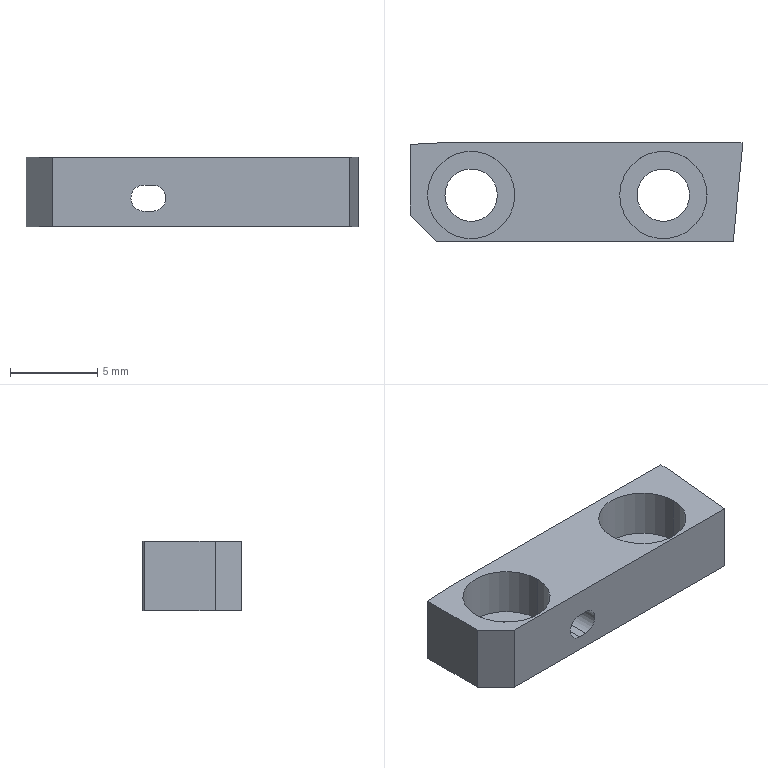Part | NX | 1 solid | 24 faces | box 19 x 5.65 x 4 mm | volume 278.189 mm3 | plane 13 | cylinder 11 | commonest cylinder face diameters 3 x4 5 x4 1.5 x3
STEP:
#1=CARTESIAN_POINT('',(18.5,0.,4.));
#2=VERTEX_POINT('',#1);
#3=CARTESIAN_POINT('',(18.5,0.,0.));
#4=VERTEX_POINT('',#3);
#5=CARTESIAN_POINT('',(18.5,0.,0.));
#6=DIRECTION('',(0.,0.,-1.));
#7=VECTOR('',#6,1000.);
#8=LINE('',#5,#7);
#9=EDGE_CURVE('',#2,#4,#8,.T.);
#10=ORIENTED_EDGE('',*,*,#9,.F.);
#11=CARTESIAN_POINT('',(1.5,0.,4.));
#12=VERTEX_POINT('',#11);
#13=CARTESIAN_POINT('',(0.,0.,4.));
#14=DIRECTION('',(-1.,0.,0.));
#15=VECTOR('',#14,1000.);
#16=LINE('',#13,#15);
#17=EDGE_CURVE('',#2,#12,#16,.T.);
#18=ORIENTED_EDGE('',*,*,#17,.T.);
#19=CARTESIAN_POINT('',(1.5,0.,0.));
#20=VERTEX_POINT('',#19);
#21=CARTESIAN_POINT('',(1.5,0.,0.));
#22=DIRECTION('',(0.,0.,1.));
#23=VECTOR('',#22,1000.);
#24=LINE('',#21,#23);
#25=EDGE_CURVE('',#20,#12,#24,.T.);
#26=ORIENTED_EDGE('',*,*,#25,.F.);
#27=CARTESIAN_POINT('',(0.,0.,0.));
#28=DIRECTION('',(1.,0.,0.));
#29=VECTOR('',#28,1000.);
#30=LINE('',#27,#29);
#31=EDGE_CURVE('',#20,#4,#30,.T.);
#32=ORIENTED_EDGE('',*,*,#31,.T.);
#33=EDGE_LOOP('',(#10,#18,#26,#32));
#34=FACE_BOUND('',#33,.T.);
#35=CARTESIAN_POINT('',(7.25,0.,2.4));
#36=VERTEX_POINT('',#35);
#37=CARTESIAN_POINT('',(7.25,0.,0.9));
#38=VERTEX_POINT('',#37);
#39=CARTESIAN_POINT('',(7.25,0.,1.65));
#40=DIRECTION('',(0.,1.,0.));
#41=DIRECTION('',(-1.,0.,0.));
#42=AXIS2_PLACEMENT_3D('',#39,#40,#41);
#43=CIRCLE('',#42,0.75);
#44=EDGE_CURVE('',#36,#38,#43,.T.);
#45=ORIENTED_EDGE('',*,*,#44,.T.);
#46=CARTESIAN_POINT('',(6.75,0.,0.9));
#47=VERTEX_POINT('',#46);
#48=CARTESIAN_POINT('',(0.,0.,0.9));
#49=DIRECTION('',(-1.,0.,0.));
#50=VECTOR('',#49,1000.);
#51=LINE('',#48,#50);
#52=EDGE_CURVE('',#38,#47,#51,.T.);
#53=ORIENTED_EDGE('',*,*,#52,.T.);
#54=CARTESIAN_POINT('',(6.,0.,1.65));
#55=VERTEX_POINT('',#54);
#56=CARTESIAN_POINT('',(6.75,0.,1.65));
#57=DIRECTION('',(0.,1.,0.));
#58=DIRECTION('',(-1.,0.,0.));
#59=AXIS2_PLACEMENT_3D('',#56,#57,#58);
#60=CIRCLE('',#59,0.75);
#61=EDGE_CURVE('',#47,#55,#60,.T.);
#62=ORIENTED_EDGE('',*,*,#61,.T.);
#63=CARTESIAN_POINT('',(6.75,0.,2.4));
#64=VERTEX_POINT('',#63);
#65=CARTESIAN_POINT('',(6.75,0.,1.65));
#66=DIRECTION('',(0.,1.,0.));
#67=DIRECTION('',(-1.,0.,0.));
#68=AXIS2_PLACEMENT_3D('',#65,#66,#67);
#69=CIRCLE('',#68,0.75);
#70=EDGE_CURVE('',#55,#64,#69,.T.);
#71=ORIENTED_EDGE('',*,*,#70,.T.);
#72=CARTESIAN_POINT('',(0.,0.,2.4));
#73=DIRECTION('',(1.,0.,0.));
#74=VECTOR('',#73,1000.);
#75=LINE('',#72,#74);
#76=EDGE_CURVE('',#64,#36,#75,.T.);
#77=ORIENTED_EDGE('',*,*,#76,.T.);
#78=EDGE_LOOP('',(#45,#53,#62,#71,#77));
#79=FACE_BOUND('',#78,.T.);
#80=CARTESIAN_POINT('',(0.,0.,0.));
#81=DIRECTION('',(0.,-1.,0.));
#82=DIRECTION('',(0.,0.,-1.));
#83=AXIS2_PLACEMENT_3D('',#80,#81,#82);
#84=PLANE('',#83);
#85=ADVANCED_FACE('',(#34,#79),#84,.T.);
#86=CARTESIAN_POINT('',(19.,5.15,0.));
#87=VERTEX_POINT('',#86);
#88=CARTESIAN_POINT('',(18.5,0.,0.));
#89=DIRECTION('',(-0.09663,-0.9953,0.));
#90=VECTOR('',#89,1000.);
#91=LINE('',#88,#90);
#92=EDGE_CURVE('',#87,#4,#91,.T.);
#93=ORIENTED_EDGE('',*,*,#92,.T.);
#94=ORIENTED_EDGE('',*,*,#31,.F.);
#95=CARTESIAN_POINT('',(0.,1.5,0.));
#96=VERTEX_POINT('',#95);
#97=CARTESIAN_POINT('',(1.5,0.,0.));
#98=DIRECTION('',(0.7071,-0.7071,0.));
#99=VECTOR('',#98,1000.);
#100=LINE('',#97,#99);
#101=EDGE_CURVE('',#96,#20,#100,.T.);
#102=ORIENTED_EDGE('',*,*,#101,.F.);
#103=CARTESIAN_POINT('',(0.,5.545,0.));
#104=VERTEX_POINT('',#103);
#105=CARTESIAN_POINT('',(0.,0.,0.));
#106=DIRECTION('',(0.,-1.,0.));
#107=VECTOR('',#106,1000.);
#108=LINE('',#105,#107);
#109=EDGE_CURVE('',#104,#96,#108,.T.);
#110=ORIENTED_EDGE('',*,*,#109,.F.);
#111=CARTESIAN_POINT('',(2.,5.65,0.));
#112=VERTEX_POINT('',#111);
#113=CARTESIAN_POINT('',(0.,5.545,0.));
#114=DIRECTION('',(-0.9986,-0.05234,0.));
#115=VECTOR('',#114,1000.);
#116=LINE('',#113,#115);
#117=EDGE_CURVE('',#112,#104,#116,.T.);
#118=ORIENTED_EDGE('',*,*,#117,.F.);
#119=CARTESIAN_POINT('',(19.,5.65,0.));
#120=VERTEX_POINT('',#119);
#121=CARTESIAN_POINT('',(0.,5.65,0.));
#122=DIRECTION('',(-1.,0.,0.));
#123=VECTOR('',#122,1000.);
#124=LINE('',#121,#123);
#125=EDGE_CURVE('',#120,#112,#124,.T.);
#126=ORIENTED_EDGE('',*,*,#125,.F.);
#127=CARTESIAN_POINT('',(19.,0.,0.));
#128=DIRECTION('',(0.,1.,0.));
#129=VECTOR('',#128,1000.);
#130=LINE('',#127,#129);
#131=EDGE_CURVE('',#87,#120,#130,.T.);
#132=ORIENTED_EDGE('',*,*,#131,.F.);
#133=EDGE_LOOP('',(#93,#94,#102,#110,#118,#126,#132));
#134=FACE_BOUND('',#133,.T.);
#135=CARTESIAN_POINT('',(2.,2.65,0.));
#136=VERTEX_POINT('',#135);
#137=CARTESIAN_POINT('',(5.,2.65,0.));
#138=VERTEX_POINT('',#137);
#139=CARTESIAN_POINT('',(3.5,2.65,0.));
#140=DIRECTION('',(0.,0.,1.));
#141=DIRECTION('',(-1.,0.,0.));
#142=AXIS2_PLACEMENT_3D('',#139,#140,#141);
#143=CIRCLE('',#142,1.5);
#144=EDGE_CURVE('',#136,#138,#143,.T.);
#145=ORIENTED_EDGE('',*,*,#144,.T.);
#146=CARTESIAN_POINT('',(3.5,2.65,0.));
#147=DIRECTION('',(0.,0.,1.));
#148=DIRECTION('',(-1.,0.,0.));
#149=AXIS2_PLACEMENT_3D('',#146,#147,#148);
#150=CIRCLE('',#149,1.5);
#151=EDGE_CURVE('',#138,#136,#150,.T.);
#152=ORIENTED_EDGE('',*,*,#151,.T.);
#153=EDGE_LOOP('',(#145,#152));
#154=FACE_BOUND('',#153,.T.);
#155=CARTESIAN_POINT('',(13.,2.65,0.));
#156=VERTEX_POINT('',#155);
#157=CARTESIAN_POINT('',(16.,2.65,0.));
#158=VERTEX_POINT('',#157);
#159=CARTESIAN_POINT('',(14.5,2.65,0.));
#160=DIRECTION('',(0.,0.,1.));
#161=DIRECTION('',(-1.,0.,0.));
#162=AXIS2_PLACEMENT_3D('',#159,#160,#161);
#163=CIRCLE('',#162,1.5);
#164=EDGE_CURVE('',#156,#158,#163,.T.);
#165=ORIENTED_EDGE('',*,*,#164,.T.);
#166=CARTESIAN_POINT('',(14.5,2.65,0.));
#167=DIRECTION('',(0.,0.,1.));
#168=DIRECTION('',(-1.,0.,0.));
#169=AXIS2_PLACEMENT_3D('',#166,#167,#168);
#170=CIRCLE('',#169,1.5);
#171=EDGE_CURVE('',#158,#156,#170,.T.);
#172=ORIENTED_EDGE('',*,*,#171,.T.);
#173=EDGE_LOOP('',(#165,#172));
#174=FACE_BOUND('',#173,.T.);
#175=CARTESIAN_POINT('',(0.,0.,0.));
#176=DIRECTION('',(0.,0.,1.));
#177=DIRECTION('',(1.,0.,0.));
#178=AXIS2_PLACEMENT_3D('',#175,#176,#177);
#179=PLANE('',#178);
#180=ADVANCED_FACE('',(#134,#154,#174),#179,.F.);
#181=CARTESIAN_POINT('',(1.,2.65,4.));
#182=VERTEX_POINT('',#181);
#183=CARTESIAN_POINT('',(6.,2.65,4.));
#184=VERTEX_POINT('',#183);
#185=CARTESIAN_POINT('',(3.5,2.65,4.));
#186=DIRECTION('',(0.,0.,1.));
#187=DIRECTION('',(-1.,0.,0.));
#188=AXIS2_PLACEMENT_3D('',#185,#186,#187);
#189=CIRCLE('',#188,2.5);
#190=EDGE_CURVE('',#182,#184,#189,.T.);
#191=ORIENTED_EDGE('',*,*,#190,.T.);
#192=CARTESIAN_POINT('',(6.,2.65,1.2));
#193=VERTEX_POINT('',#192);
#194=CARTESIAN_POINT('',(6.,2.65,-0.775));
#195=DIRECTION('',(0.,0.,1.));
#196=VECTOR('',#195,1000.);
#197=LINE('',#194,#196);
#198=EDGE_CURVE('',#193,#184,#197,.T.);
#199=ORIENTED_EDGE('',*,*,#198,.F.);
#200=CARTESIAN_POINT('',(1.,2.65,1.2));
#201=VERTEX_POINT('',#200);
#202=CARTESIAN_POINT('',(3.5,2.65,1.2));
#203=DIRECTION('',(0.,0.,1.));
#204=DIRECTION('',(-1.,0.,0.));
#205=AXIS2_PLACEMENT_3D('',#202,#203,#204);
#206=CIRCLE('',#205,2.5);
#207=EDGE_CURVE('',#201,#193,#206,.T.);
#208=ORIENTED_EDGE('',*,*,#207,.F.);
#209=CARTESIAN_POINT('',(1.,2.65,-0.775));
#210=DIRECTION('',(0.,0.,1.));
#211=VECTOR('',#210,1000.);
#212=LINE('',#209,#211);
#213=EDGE_CURVE('',#201,#182,#212,.T.);
#214=ORIENTED_EDGE('',*,*,#213,.T.);
#215=EDGE_LOOP('',(#191,#199,#208,#214));
#216=FACE_BOUND('',#215,.T.);
#217=CARTESIAN_POINT('',(3.5,2.65,-0.775));
#218=DIRECTION('',(0.,0.,1.));
#219=DIRECTION('',(-1.,0.,0.));
#220=AXIS2_PLACEMENT_3D('',#217,#218,#219);
#221=CYLINDRICAL_SURFACE('',#220,2.5);
#222=ADVANCED_FACE('',(#216),#221,.F.);
#223=ORIENTED_EDGE('',*,*,#109,.T.);
#224=CARTESIAN_POINT('',(0.,1.5,4.));
#225=VERTEX_POINT('',#224);
#226=CARTESIAN_POINT('',(0.,1.5,0.));
#227=DIRECTION('',(0.,0.,1.));
#228=VECTOR('',#227,1000.);
#229=LINE('',#226,#228);
#230=EDGE_CURVE('',#96,#225,#229,.T.);
#231=ORIENTED_EDGE('',*,*,#230,.T.);
#232=CARTESIAN_POINT('',(0.,5.545,4.));
#233=VERTEX_POINT('',#232);
#234=CARTESIAN_POINT('',(0.,0.,4.));
#235=DIRECTION('',(0.,1.,0.));
#236=VECTOR('',#235,1000.);
#237=LINE('',#234,#236);
#238=EDGE_CURVE('',#225,#233,#237,.T.);
#239=ORIENTED_EDGE('',*,*,#238,.T.);
#240=CARTESIAN_POINT('',(0.,5.545,0.));
#241=DIRECTION('',(0.,0.,1.));
#242=VECTOR('',#241,1000.);
#243=LINE('',#240,#242);
#244=EDGE_CURVE('',#104,#233,#243,.T.);
#245=ORIENTED_EDGE('',*,*,#244,.F.);
#246=EDGE_LOOP('',(#223,#231,#239,#245));
#247=FACE_BOUND('',#246,.T.);
#248=CARTESIAN_POINT('',(0.,5.65,0.));
#249=DIRECTION('',(-1.,0.,0.));
#250=DIRECTION('',(0.,0.,1.));
#251=AXIS2_PLACEMENT_3D('',#248,#249,#250);
#252=PLANE('',#251);
#253=ADVANCED_FACE('',(#247),#252,.T.);
#254=CARTESIAN_POINT('',(1.5,0.,4.));
#255=DIRECTION('',(-0.7071,0.7071,0.));
#256=VECTOR('',#255,1000.);
#257=LINE('',#254,#256);
#258=EDGE_CURVE('',#12,#225,#257,.T.);
#259=ORIENTED_EDGE('',*,*,#258,.T.);
#260=ORIENTED_EDGE('',*,*,#230,.F.);
#261=ORIENTED_EDGE('',*,*,#101,.T.);
#262=ORIENTED_EDGE('',*,*,#25,.T.);
#263=EDGE_LOOP('',(#259,#260,#261,#262));
#264=FACE_BOUND('',#263,.T.);
#265=CARTESIAN_POINT('',(1.5,0.,0.));
#266=DIRECTION('',(-0.7071,-0.7071,0.));
#267=DIRECTION('',(-0.7071,0.7071,0.));
#268=AXIS2_PLACEMENT_3D('',#265,#266,#267);
#269=PLANE('',#268);
#270=ADVANCED_FACE('',(#264),#269,.T.);
#271=ORIENTED_EDGE('',*,*,#92,.F.);
#272=CARTESIAN_POINT('',(19.,5.15,4.));
#273=VERTEX_POINT('',#272);
#274=CARTESIAN_POINT('',(19.,5.15,0.));
#275=DIRECTION('',(0.,0.,1.));
#276=VECTOR('',#275,1000.);
#277=LINE('',#274,#276);
#278=EDGE_CURVE('',#87,#273,#277,.T.);
#279=ORIENTED_EDGE('',*,*,#278,.T.);
#280=CARTESIAN_POINT('',(18.5,0.,4.));
#281=DIRECTION('',(0.09663,0.9953,0.));
#282=VECTOR('',#281,1000.);
#283=LINE('',#280,#282);
#284=EDGE_CURVE('',#2,#273,#283,.T.);
#285=ORIENTED_EDGE('',*,*,#284,.F.);
#286=ORIENTED_EDGE('',*,*,#9,.T.);
#287=EDGE_LOOP('',(#271,#279,#285,#286));
#288=FACE_BOUND('',#287,.T.);
#289=CARTESIAN_POINT('',(18.5,0.,-0.45));
#290=DIRECTION('',(-0.9953,0.09663,0.));
#291=DIRECTION('',(0.,0.,1.));
#292=AXIS2_PLACEMENT_3D('',#289,#290,#291);
#293=PLANE('',#292);
#294=ADVANCED_FACE('',(#288),#293,.F.);
#295=ORIENTED_EDGE('',*,*,#131,.T.);
#296=CARTESIAN_POINT('',(19.,5.65,4.));
#297=VERTEX_POINT('',#296);
#298=CARTESIAN_POINT('',(19.,5.65,0.));
#299=DIRECTION('',(0.,0.,1.));
#300=VECTOR('',#299,1000.);
#301=LINE('',#298,#300);
#302=EDGE_CURVE('',#120,#297,#301,.T.);
#303=ORIENTED_EDGE('',*,*,#302,.T.);
#304=CARTESIAN_POINT('',(19.,0.,4.));
#305=DIRECTION('',(0.,-1.,0.));
#306=VECTOR('',#305,1000.);
#307=LINE('',#304,#306);
#308=EDGE_CURVE('',#297,#273,#307,.T.);
#309=ORIENTED_EDGE('',*,*,#308,.T.);
#310=ORIENTED_EDGE('',*,*,#278,.F.);
#311=EDGE_LOOP('',(#295,#303,#309,#310));
#312=FACE_BOUND('',#311,.T.);
#313=CARTESIAN_POINT('',(19.,0.,0.));
#314=DIRECTION('',(1.,0.,0.));
#315=DIRECTION('',(0.,1.,0.));
#316=AXIS2_PLACEMENT_3D('',#313,#314,#315);
#317=PLANE('',#316);
#318=ADVANCED_FACE('',(#312),#317,.T.);
#319=CARTESIAN_POINT('',(6.,5.65,1.65));
#320=VERTEX_POINT('',#319);
#321=CARTESIAN_POINT('',(6.,-0.565,1.65));
#322=DIRECTION('',(0.,1.,0.));
#323=VECTOR('',#322,1000.);
#324=LINE('',#321,#323);
#325=EDGE_CURVE('',#55,#320,#324,.T.);
#326=ORIENTED_EDGE('',*,*,#325,.F.);
#327=ORIENTED_EDGE('',*,*,#61,.F.);
#328=CARTESIAN_POINT('',(6.75,5.65,0.9));
#329=VERTEX_POINT('',#328);
#330=CARTESIAN_POINT('',(6.75,-0.565,0.9));
#331=DIRECTION('',(0.,1.,0.));
#332=VECTOR('',#331,1000.);
#333=LINE('',#330,#332);
#334=EDGE_CURVE('',#47,#329,#333,.T.);
#335=ORIENTED_EDGE('',*,*,#334,.T.);
#336=CARTESIAN_POINT('',(6.75,5.65,1.65));
#337=DIRECTION('',(0.,1.,0.));
#338=DIRECTION('',(-1.,0.,0.));
#339=AXIS2_PLACEMENT_3D('',#336,#337,#338);
#340=CIRCLE('',#339,0.75);
#341=EDGE_CURVE('',#329,#320,#340,.T.);
#342=ORIENTED_EDGE('',*,*,#341,.T.);
#343=EDGE_LOOP('',(#326,#327,#335,#342));
#344=FACE_BOUND('',#343,.T.);
#345=CARTESIAN_POINT('',(6.75,-0.565,1.65));
#346=DIRECTION('',(0.,1.,0.));
#347=DIRECTION('',(-1.,0.,0.));
#348=AXIS2_PLACEMENT_3D('',#345,#346,#347);
#349=CYLINDRICAL_SURFACE('',#348,0.75);
#350=ADVANCED_FACE('',(#344),#349,.F.);
#351=CARTESIAN_POINT('',(12.,2.65,1.2));
#352=VERTEX_POINT('',#351);
#353=CARTESIAN_POINT('',(17.,2.65,1.2));
#354=VERTEX_POINT('',#353);
#355=CARTESIAN_POINT('',(14.5,2.65,1.2));
#356=DIRECTION('',(0.,0.,1.));
#357=DIRECTION('',(-1.,0.,0.));
#358=AXIS2_PLACEMENT_3D('',#355,#356,#357);
#359=CIRCLE('',#358,2.5);
#360=EDGE_CURVE('',#352,#354,#359,.T.);
#361=ORIENTED_EDGE('',*,*,#360,.T.);
#362=CARTESIAN_POINT('',(14.5,2.65,1.2));
#363=DIRECTION('',(0.,0.,1.));
#364=DIRECTION('',(-1.,0.,0.));
#365=AXIS2_PLACEMENT_3D('',#362,#363,#364);
#366=CIRCLE('',#365,2.5);
#367=EDGE_CURVE('',#354,#352,#366,.T.);
#368=ORIENTED_EDGE('',*,*,#367,.T.);
#369=EDGE_LOOP('',(#361,#368));
#370=FACE_BOUND('',#369,.T.);
#371=CARTESIAN_POINT('',(16.,2.65,1.2));
#372=VERTEX_POINT('',#371);
#373=CARTESIAN_POINT('',(13.,2.65,1.2));
#374=VERTEX_POINT('',#373);
#375=CARTESIAN_POINT('',(14.5,2.65,1.2));
#376=DIRECTION('',(0.,0.,1.));
#377=DIRECTION('',(-1.,0.,0.));
#378=AXIS2_PLACEMENT_3D('',#375,#376,#377);
#379=CIRCLE('',#378,1.5);
#380=EDGE_CURVE('',#372,#374,#379,.T.);
#381=ORIENTED_EDGE('',*,*,#380,.F.);
#382=CARTESIAN_POINT('',(14.5,2.65,1.2));
#383=DIRECTION('',(0.,0.,1.));
#384=DIRECTION('',(-1.,0.,0.));
#385=AXIS2_PLACEMENT_3D('',#382,#383,#384);
#386=CIRCLE('',#385,1.5);
#387=EDGE_CURVE('',#374,#372,#386,.T.);
#388=ORIENTED_EDGE('',*,*,#387,.F.);
#389=EDGE_LOOP('',(#381,#388));
#390=FACE_BOUND('',#389,.T.);
#391=CARTESIAN_POINT('',(14.5,2.65,1.2));
#392=DIRECTION('',(0.,0.,1.));
#393=DIRECTION('',(1.,0.,0.));
#394=AXIS2_PLACEMENT_3D('',#391,#392,#393);
#395=PLANE('',#394);
#396=ADVANCED_FACE('',(#370,#390),#395,.T.);
#397=CARTESIAN_POINT('',(7.25,5.65,2.4));
#398=VERTEX_POINT('',#397);
#399=CARTESIAN_POINT('',(6.75,5.65,2.4));
#400=VERTEX_POINT('',#399);
#401=CARTESIAN_POINT('',(0.,5.65,2.4));
#402=DIRECTION('',(-1.,0.,0.));
#403=VECTOR('',#402,1000.);
#404=LINE('',#401,#403);
#405=EDGE_CURVE('',#398,#400,#404,.T.);
#406=ORIENTED_EDGE('',*,*,#405,.F.);
#407=CARTESIAN_POINT('',(7.25,-0.565,2.4));
#408=DIRECTION('',(0.,1.,0.));
#409=VECTOR('',#408,1000.);
#410=LINE('',#407,#409);
#411=EDGE_CURVE('',#36,#398,#410,.T.);
#412=ORIENTED_EDGE('',*,*,#411,.F.);
#413=ORIENTED_EDGE('',*,*,#76,.F.);
#414=CARTESIAN_POINT('',(6.75,-0.565,2.4));
#415=DIRECTION('',(0.,1.,0.));
#416=VECTOR('',#415,1000.);
#417=LINE('',#414,#416);
#418=EDGE_CURVE('',#64,#400,#417,.T.);
#419=ORIENTED_EDGE('',*,*,#418,.T.);
#420=EDGE_LOOP('',(#406,#412,#413,#419));
#421=FACE_BOUND('',#420,.T.);
#422=CARTESIAN_POINT('',(7.25,-0.565,2.4));
#423=DIRECTION('',(0.,0.,1.));
#424=DIRECTION('',(1.,0.,0.));
#425=AXIS2_PLACEMENT_3D('',#422,#423,#424);
#426=PLANE('',#425);
#427=ADVANCED_FACE('',(#421),#426,.F.);
#428=ORIENTED_EDGE('',*,*,#125,.T.);
#429=CARTESIAN_POINT('',(2.,5.65,4.));
#430=VERTEX_POINT('',#429);
#431=CARTESIAN_POINT('',(2.,5.65,0.));
#432=DIRECTION('',(0.,0.,-1.));
#433=VECTOR('',#432,1000.);
#434=LINE('',#431,#433);
#435=EDGE_CURVE('',#430,#112,#434,.T.);
#436=ORIENTED_EDGE('',*,*,#435,.F.);
#437=CARTESIAN_POINT('',(0.,5.65,4.));
#438=DIRECTION('',(1.,0.,0.));
#439=VECTOR('',#438,1000.);
#440=LINE('',#437,#439);
#441=EDGE_CURVE('',#430,#297,#440,.T.);
#442=ORIENTED_EDGE('',*,*,#441,.T.);
#443=ORIENTED_EDGE('',*,*,#302,.F.);
#444=EDGE_LOOP('',(#428,#436,#442,#443));
#445=FACE_BOUND('',#444,.T.);
#446=CARTESIAN_POINT('',(7.25,5.65,0.9));
#447=VERTEX_POINT('',#446);
#448=CARTESIAN_POINT('',(0.,5.65,0.9));
#449=DIRECTION('',(1.,0.,0.));
#450=VECTOR('',#449,1000.);
#451=LINE('',#448,#450);
#452=EDGE_CURVE('',#329,#447,#451,.T.);
#453=ORIENTED_EDGE('',*,*,#452,.T.);
#454=CARTESIAN_POINT('',(7.25,5.65,1.65));
#455=DIRECTION('',(0.,1.,0.));
#456=DIRECTION('',(-1.,0.,0.));
#457=AXIS2_PLACEMENT_3D('',#454,#455,#456);
#458=CIRCLE('',#457,0.75);
#459=EDGE_CURVE('',#398,#447,#458,.T.);
#460=ORIENTED_EDGE('',*,*,#459,.F.);
#461=ORIENTED_EDGE('',*,*,#405,.T.);
#462=CARTESIAN_POINT('',(6.75,5.65,1.65));
#463=DIRECTION('',(0.,1.,0.));
#464=DIRECTION('',(-1.,0.,0.));
#465=AXIS2_PLACEMENT_3D('',#462,#463,#464);
#466=CIRCLE('',#465,0.75);
#467=EDGE_CURVE('',#320,#400,#466,.T.);
#468=ORIENTED_EDGE('',*,*,#467,.F.);
#469=ORIENTED_EDGE('',*,*,#341,.F.);
#470=EDGE_LOOP('',(#453,#460,#461,#468,#469));
#471=FACE_BOUND('',#470,.T.);
#472=CARTESIAN_POINT('',(19.,5.65,0.));
#473=DIRECTION('',(0.,1.,0.));
#474=DIRECTION('',(1.,0.,0.));
#475=AXIS2_PLACEMENT_3D('',#472,#473,#474);
#476=PLANE('',#475);
#477=ADVANCED_FACE('',(#445,#471),#476,.T.);
#478=ORIENTED_EDGE('',*,*,#144,.F.);
#479=CARTESIAN_POINT('',(2.,2.65,1.2));
#480=VERTEX_POINT('',#479);
#481=CARTESIAN_POINT('',(2.,2.65,-0.775));
#482=DIRECTION('',(0.,0.,1.));
#483=VECTOR('',#482,1000.);
#484=LINE('',#481,#483);
#485=EDGE_CURVE('',#480,#136,#484,.F.);
#486=ORIENTED_EDGE('',*,*,#485,.F.);
#487=CARTESIAN_POINT('',(5.,2.65,1.2));
#488=VERTEX_POINT('',#487);
#489=CARTESIAN_POINT('',(3.5,2.65,1.2));
#490=DIRECTION('',(0.,0.,1.));
#491=DIRECTION('',(-1.,0.,0.));
#492=AXIS2_PLACEMENT_3D('',#489,#490,#491);
#493=CIRCLE('',#492,1.5);
#494=EDGE_CURVE('',#480,#488,#493,.T.);
#495=ORIENTED_EDGE('',*,*,#494,.T.);
#496=CARTESIAN_POINT('',(5.,2.65,-0.775));
#497=DIRECTION('',(0.,0.,1.));
#498=VECTOR('',#497,1000.);
#499=LINE('',#496,#498);
#500=EDGE_CURVE('',#488,#138,#499,.F.);
#501=ORIENTED_EDGE('',*,*,#500,.T.);
#502=EDGE_LOOP('',(#478,#486,#495,#501));
#503=FACE_BOUND('',#502,.T.);
#504=CARTESIAN_POINT('',(3.5,2.65,-0.775));
#505=DIRECTION('',(0.,0.,1.));
#506=DIRECTION('',(-1.,0.,0.));
#507=AXIS2_PLACEMENT_3D('',#504,#505,#506);
#508=CYLINDRICAL_SURFACE('',#507,1.5);
#509=ADVANCED_FACE('',(#503),#508,.F.);
#510=ORIENTED_EDGE('',*,*,#459,.T.);
#511=CARTESIAN_POINT('',(7.25,-0.565,0.9));
#512=DIRECTION('',(0.,1.,0.));
#513=VECTOR('',#512,1000.);
#514=LINE('',#511,#513);
#515=EDGE_CURVE('',#38,#447,#514,.T.);
#516=ORIENTED_EDGE('',*,*,#515,.F.);
#517=ORIENTED_EDGE('',*,*,#44,.F.);
#518=ORIENTED_EDGE('',*,*,#411,.T.);
#519=EDGE_LOOP('',(#510,#516,#517,#518));
#520=FACE_BOUND('',#519,.T.);
#521=CARTESIAN_POINT('',(7.25,-0.565,1.65));
#522=DIRECTION('',(0.,1.,0.));
#523=DIRECTION('',(-1.,0.,0.));
#524=AXIS2_PLACEMENT_3D('',#521,#522,#523);
#525=CYLINDRICAL_SURFACE('',#524,0.75);
#526=ADVANCED_FACE('',(#520),#525,.F.);
#527=ORIENTED_EDGE('',*,*,#360,.F.);
#528=CARTESIAN_POINT('',(12.,2.65,4.));
#529=VERTEX_POINT('',#528);
#530=CARTESIAN_POINT('',(12.,2.65,-0.775));
#531=DIRECTION('',(0.,0.,1.));
#532=VECTOR('',#531,1000.);
#533=LINE('',#530,#532);
#534=EDGE_CURVE('',#529,#352,#533,.F.);
#535=ORIENTED_EDGE('',*,*,#534,.F.);
#536=CARTESIAN_POINT('',(17.,2.65,4.));
#537=VERTEX_POINT('',#536);
#538=CARTESIAN_POINT('',(14.5,2.65,4.));
#539=DIRECTION('',(0.,0.,1.));
#540=DIRECTION('',(-1.,0.,0.));
#541=AXIS2_PLACEMENT_3D('',#538,#539,#540);
#542=CIRCLE('',#541,2.5);
#543=EDGE_CURVE('',#529,#537,#542,.T.);
#544=ORIENTED_EDGE('',*,*,#543,.T.);
#545=CARTESIAN_POINT('',(17.,2.65,-0.775));
#546=DIRECTION('',(0.,0.,1.));
#547=VECTOR('',#546,1000.);
#548=LINE('',#545,#547);
#549=EDGE_CURVE('',#537,#354,#548,.F.);
#550=ORIENTED_EDGE('',*,*,#549,.T.);
#551=EDGE_LOOP('',(#527,#535,#544,#550));
#552=FACE_BOUND('',#551,.T.);
#553=CARTESIAN_POINT('',(14.5,2.65,-0.775));
#554=DIRECTION('',(0.,0.,1.));
#555=DIRECTION('',(-1.,0.,0.));
#556=AXIS2_PLACEMENT_3D('',#553,#554,#555);
#557=CYLINDRICAL_SURFACE('',#556,2.5);
#558=ADVANCED_FACE('',(#552),#557,.F.);
#559=ORIENTED_EDGE('',*,*,#52,.F.);
#560=ORIENTED_EDGE('',*,*,#515,.T.);
#561=ORIENTED_EDGE('',*,*,#452,.F.);
#562=ORIENTED_EDGE('',*,*,#334,.F.);
#563=EDGE_LOOP('',(#559,#560,#561,#562));
#564=FACE_BOUND('',#563,.T.);
#565=CARTESIAN_POINT('',(6.75,-0.565,0.9));
#566=DIRECTION('',(0.,0.,-1.));
#567=DIRECTION('',(0.,-1.,0.));
#568=AXIS2_PLACEMENT_3D('',#565,#566,#567);
#569=PLANE('',#568);
#570=ADVANCED_FACE('',(#564),#569,.F.);
#571=CARTESIAN_POINT('',(0.,5.545,4.));
#572=DIRECTION('',(0.9986,0.05234,0.));
#573=VECTOR('',#572,1000.);
#574=LINE('',#571,#573);
#575=EDGE_CURVE('',#233,#430,#574,.T.);
#576=ORIENTED_EDGE('',*,*,#575,.T.);
#577=ORIENTED_EDGE('',*,*,#435,.T.);
#578=ORIENTED_EDGE('',*,*,#117,.T.);
#579=ORIENTED_EDGE('',*,*,#244,.T.);
#580=EDGE_LOOP('',(#576,#577,#578,#579));
#581=FACE_BOUND('',#580,.T.);
#582=CARTESIAN_POINT('',(0.,5.545,0.));
#583=DIRECTION('',(-0.05234,0.9986,0.));
#584=DIRECTION('',(0.,0.,1.));
#585=AXIS2_PLACEMENT_3D('',#582,#583,#584);
#586=PLANE('',#585);
#587=ADVANCED_FACE('',(#581),#586,.T.);
#588=ORIENTED_EDGE('',*,*,#164,.F.);
#589=CARTESIAN_POINT('',(13.,2.65,-0.775));
#590=DIRECTION('',(0.,0.,1.));
#591=VECTOR('',#590,1000.);
#592=LINE('',#589,#591);
#593=EDGE_CURVE('',#374,#156,#592,.F.);
#594=ORIENTED_EDGE('',*,*,#593,.F.);
#595=ORIENTED_EDGE('',*,*,#387,.T.);
#596=CARTESIAN_POINT('',(16.,2.65,-0.775));
#597=DIRECTION('',(0.,0.,1.));
#598=VECTOR('',#597,1000.);
#599=LINE('',#596,#598);
#600=EDGE_CURVE('',#372,#158,#599,.F.);
#601=ORIENTED_EDGE('',*,*,#600,.T.);
#602=EDGE_LOOP('',(#588,#594,#595,#601));
#603=FACE_BOUND('',#602,.T.);
#604=CARTESIAN_POINT('',(14.5,2.65,-0.775));
#605=DIRECTION('',(0.,0.,1.));
#606=DIRECTION('',(-1.,0.,0.));
#607=AXIS2_PLACEMENT_3D('',#604,#605,#606);
#608=CYLINDRICAL_SURFACE('',#607,1.5);
#609=ADVANCED_FACE('',(#603),#608,.F.);
#610=CARTESIAN_POINT('',(3.5,2.65,1.2));
#611=DIRECTION('',(0.,0.,1.));
#612=DIRECTION('',(-1.,0.,0.));
#613=AXIS2_PLACEMENT_3D('',#610,#611,#612);
#614=CIRCLE('',#613,2.5);
#615=EDGE_CURVE('',#193,#201,#614,.T.);
#616=ORIENTED_EDGE('',*,*,#615,.T.);
#617=ORIENTED_EDGE('',*,*,#207,.T.);
#618=EDGE_LOOP('',(#616,#617));
#619=FACE_BOUND('',#618,.T.);
#620=ORIENTED_EDGE('',*,*,#494,.F.);
#621=CARTESIAN_POINT('',(3.5,2.65,1.2));
#622=DIRECTION('',(0.,0.,1.));
#623=DIRECTION('',(-1.,0.,0.));
#624=AXIS2_PLACEMENT_3D('',#621,#622,#623);
#625=CIRCLE('',#624,1.5);
#626=EDGE_CURVE('',#488,#480,#625,.T.);
#627=ORIENTED_EDGE('',*,*,#626,.F.);
#628=EDGE_LOOP('',(#620,#627));
#629=FACE_BOUND('',#628,.T.);
#630=CARTESIAN_POINT('',(3.5,2.65,1.2));
#631=DIRECTION('',(0.,0.,1.));
#632=DIRECTION('',(1.,0.,0.));
#633=AXIS2_PLACEMENT_3D('',#630,#631,#632);
#634=PLANE('',#633);
#635=ADVANCED_FACE('',(#619,#629),#634,.T.);
#636=ORIENTED_EDGE('',*,*,#308,.F.);
#637=ORIENTED_EDGE('',*,*,#441,.F.);
#638=ORIENTED_EDGE('',*,*,#575,.F.);
#639=ORIENTED_EDGE('',*,*,#238,.F.);
#640=ORIENTED_EDGE('',*,*,#258,.F.);
#641=ORIENTED_EDGE('',*,*,#17,.F.);
#642=ORIENTED_EDGE('',*,*,#284,.T.);
#643=EDGE_LOOP('',(#636,#637,#638,#639,#640,#641,#642));
#644=FACE_BOUND('',#643,.T.);
#645=ORIENTED_EDGE('',*,*,#543,.F.);
#646=CARTESIAN_POINT('',(14.5,2.65,4.));
#647=DIRECTION('',(0.,0.,1.));
#648=DIRECTION('',(-1.,0.,0.));
#649=AXIS2_PLACEMENT_3D('',#646,#647,#648);
#650=CIRCLE('',#649,2.5);
#651=EDGE_CURVE('',#537,#529,#650,.T.);
#652=ORIENTED_EDGE('',*,*,#651,.F.);
#653=EDGE_LOOP('',(#645,#652));
#654=FACE_BOUND('',#653,.T.);
#655=ORIENTED_EDGE('',*,*,#190,.F.);
#656=CARTESIAN_POINT('',(3.5,2.65,4.));
#657=DIRECTION('',(0.,0.,1.));
#658=DIRECTION('',(-1.,0.,0.));
#659=AXIS2_PLACEMENT_3D('',#656,#657,#658);
#660=CIRCLE('',#659,2.5);
#661=EDGE_CURVE('',#184,#182,#660,.T.);
#662=ORIENTED_EDGE('',*,*,#661,.F.);
#663=EDGE_LOOP('',(#655,#662));
#664=FACE_BOUND('',#663,.T.);
#665=CARTESIAN_POINT('',(0.,0.,4.));
#666=DIRECTION('',(0.,0.,1.));
#667=DIRECTION('',(1.,0.,0.));
#668=AXIS2_PLACEMENT_3D('',#665,#666,#667);
#669=PLANE('',#668);
#670=ADVANCED_FACE('',(#644,#654,#664),#669,.T.);
#671=ORIENTED_EDGE('',*,*,#380,.T.);
#672=ORIENTED_EDGE('',*,*,#593,.T.);
#673=ORIENTED_EDGE('',*,*,#171,.F.);
#674=ORIENTED_EDGE('',*,*,#600,.F.);
#675=EDGE_LOOP('',(#671,#672,#673,#674));
#676=FACE_BOUND('',#675,.T.);
#677=CARTESIAN_POINT('',(14.5,2.65,-0.775));
#678=DIRECTION('',(0.,0.,1.));
#679=DIRECTION('',(-1.,0.,0.));
#680=AXIS2_PLACEMENT_3D('',#677,#678,#679);
#681=CYLINDRICAL_SURFACE('',#680,1.5);
#682=ADVANCED_FACE('',(#676),#681,.F.);
#683=ORIENTED_EDGE('',*,*,#615,.F.);
#684=ORIENTED_EDGE('',*,*,#198,.T.);
#685=ORIENTED_EDGE('',*,*,#661,.T.);
#686=ORIENTED_EDGE('',*,*,#213,.F.);
#687=EDGE_LOOP('',(#683,#684,#685,#686));
#688=FACE_BOUND('',#687,.T.);
#689=CARTESIAN_POINT('',(3.5,2.65,-0.775));
#690=DIRECTION('',(0.,0.,1.));
#691=DIRECTION('',(-1.,0.,0.));
#692=AXIS2_PLACEMENT_3D('',#689,#690,#691);
#693=CYLINDRICAL_SURFACE('',#692,2.5);
#694=ADVANCED_FACE('',(#688),#693,.F.);
#695=ORIENTED_EDGE('',*,*,#534,.T.);
#696=ORIENTED_EDGE('',*,*,#367,.F.);
#697=ORIENTED_EDGE('',*,*,#549,.F.);
#698=ORIENTED_EDGE('',*,*,#651,.T.);
#699=EDGE_LOOP('',(#695,#696,#697,#698));
#700=FACE_BOUND('',#699,.T.);
#701=CARTESIAN_POINT('',(14.5,2.65,-0.775));
#702=DIRECTION('',(0.,0.,1.));
#703=DIRECTION('',(-1.,0.,0.));
#704=AXIS2_PLACEMENT_3D('',#701,#702,#703);
#705=CYLINDRICAL_SURFACE('',#704,2.5);
#706=ADVANCED_FACE('',(#700),#705,.F.);
#707=ORIENTED_EDGE('',*,*,#485,.T.);
#708=ORIENTED_EDGE('',*,*,#151,.F.);
#709=ORIENTED_EDGE('',*,*,#500,.F.);
#710=ORIENTED_EDGE('',*,*,#626,.T.);
#711=EDGE_LOOP('',(#707,#708,#709,#710));
#712=FACE_BOUND('',#711,.T.);
#713=CARTESIAN_POINT('',(3.5,2.65,-0.775));
#714=DIRECTION('',(0.,0.,1.));
#715=DIRECTION('',(-1.,0.,0.));
#716=AXIS2_PLACEMENT_3D('',#713,#714,#715);
#717=CYLINDRICAL_SURFACE('',#716,1.5);
#718=ADVANCED_FACE('',(#712),#717,.F.);
#719=ORIENTED_EDGE('',*,*,#70,.F.);
#720=ORIENTED_EDGE('',*,*,#325,.T.);
#721=ORIENTED_EDGE('',*,*,#467,.T.);
#722=ORIENTED_EDGE('',*,*,#418,.F.);
#723=EDGE_LOOP('',(#719,#720,#721,#722));
#724=FACE_BOUND('',#723,.T.);
#725=CARTESIAN_POINT('',(6.75,-0.565,1.65));
#726=DIRECTION('',(0.,1.,0.));
#727=DIRECTION('',(-1.,0.,0.));
#728=AXIS2_PLACEMENT_3D('',#725,#726,#727);
#729=CYLINDRICAL_SURFACE('',#728,0.75);
#730=ADVANCED_FACE('',(#724),#729,.F.);
#731=CLOSED_SHELL('',(#85,#180,#222,#253,#270,#294,#318,#350,#396,#427,#477,#509,#526,#558,#570,#587,#609,#635,#670,#682,#694,#706,#718,#730));
#732=MANIFOLD_SOLID_BREP('',#731);
#733=(LENGTH_UNIT()NAMED_UNIT(*)SI_UNIT(.MILLI.,.METRE.));
#734=UNCERTAINTY_MEASURE_WITH_UNIT(LENGTH_MEASURE(0.00001),#733,'','');
#735=(NAMED_UNIT(*)PLANE_ANGLE_UNIT()SI_UNIT($,.RADIAN.));
#736=(NAMED_UNIT(*)SI_UNIT($,.STERADIAN.)SOLID_ANGLE_UNIT());
#737=(GEOMETRIC_REPRESENTATION_CONTEXT(3)GLOBAL_UNCERTAINTY_ASSIGNED_CONTEXT((#734))GLOBAL_UNIT_ASSIGNED_CONTEXT((#733,#735,#736))REPRESENTATION_CONTEXT('',''));
#738=ADVANCED_BREP_SHAPE_REPRESENTATION('',(#732),#737);